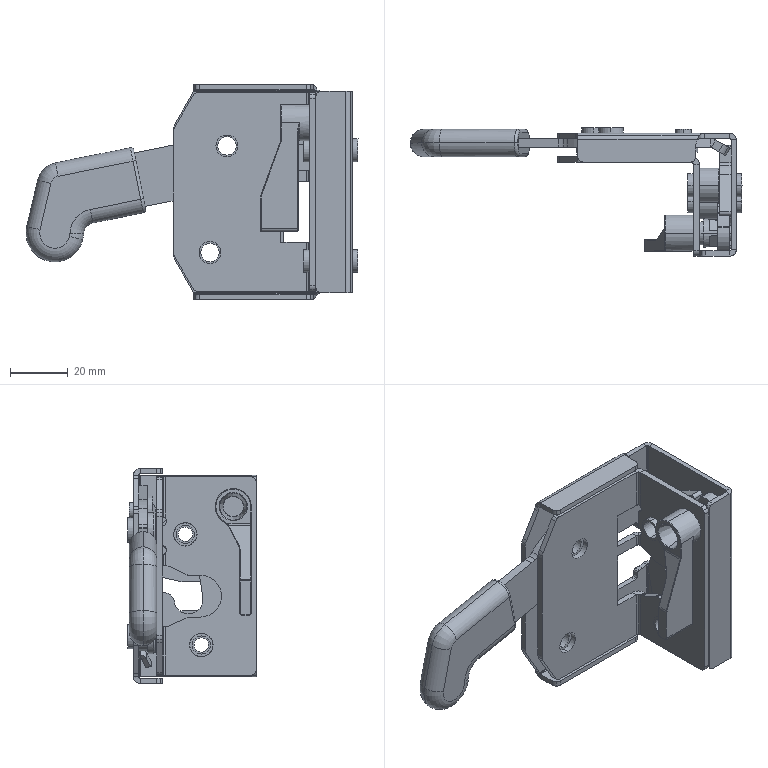Part | NX | features BREP 15 | 15 solids | 646 faces | box 115.249 x 44.6 x 74.6 mm | volume 46344 mm3 | cylinder 371 | plane 205 | torus 34 | cone 20 | spline 16 | commonest cylinder face diameters 4 x44 2 x37 10 x33 1 x27 8.1 x20 12 x20